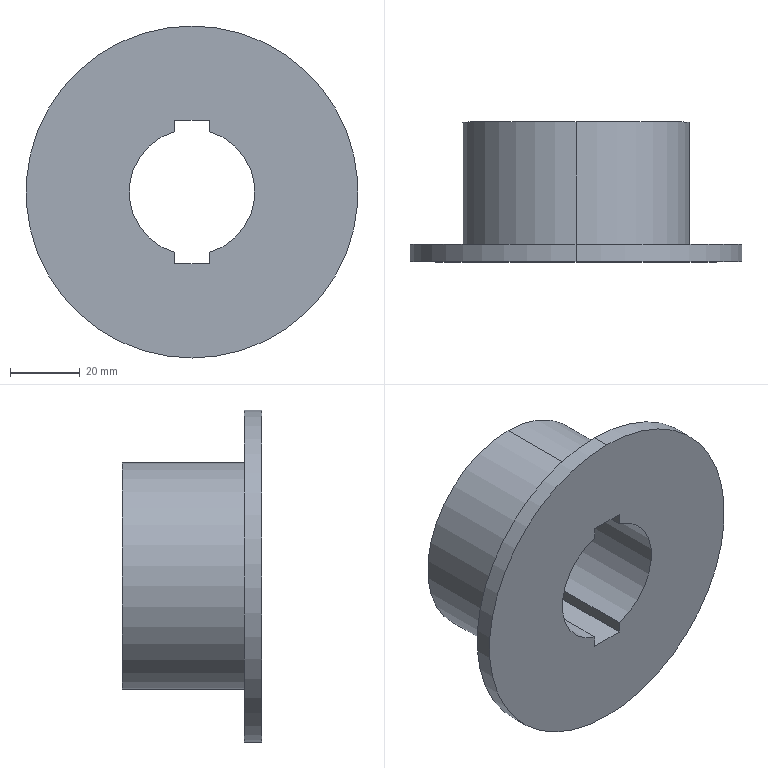Part | SolidWorks | features Extrusion 1, ICE 1 | 1 solid | 15 faces | box 95 x 40 x 95 mm | volume 108607 mm3 | plane 9 | cylinder 6 | commonest cylinder face diameters 36 x2 65 x2 95 x2
STEP:
#1=CARTESIAN_POINT('',(0.,5.,-47.5));
#2=VERTEX_POINT('',#1);
#3=CARTESIAN_POINT('',(0.,5.,47.5));
#4=VERTEX_POINT('',#3);
#5=CARTESIAN_POINT('',(0.,5.,0.));
#6=DIRECTION('',(0.,-1.,0.));
#7=DIRECTION('',(0.,0.,-1.));
#8=AXIS2_PLACEMENT_3D('',#5,#6,#7);
#9=CIRCLE('',#8,47.5);
#10=EDGE_CURVE('',#2,#4,#9,.T.);
#11=ORIENTED_EDGE('',*,*,#10,.T.);
#12=CARTESIAN_POINT('',(0.,0.,47.5));
#13=VERTEX_POINT('',#12);
#14=CARTESIAN_POINT('',(0.,5.,47.5));
#15=DIRECTION('',(0.,-1.,0.));
#16=VECTOR('',#15,1000.);
#17=LINE('',#14,#16);
#18=EDGE_CURVE('',#4,#13,#17,.T.);
#19=ORIENTED_EDGE('',*,*,#18,.T.);
#20=CARTESIAN_POINT('',(0.,0.,-47.5));
#21=VERTEX_POINT('',#20);
#22=CARTESIAN_POINT('',(0.,0.,0.));
#23=DIRECTION('',(0.,-1.,0.));
#24=DIRECTION('',(0.,0.,-1.));
#25=AXIS2_PLACEMENT_3D('',#22,#23,#24);
#26=CIRCLE('',#25,47.5);
#27=EDGE_CURVE('',#21,#13,#26,.T.);
#28=ORIENTED_EDGE('',*,*,#27,.F.);
#29=CARTESIAN_POINT('',(0.,5.,-47.5));
#30=DIRECTION('',(0.,-1.,0.));
#31=VECTOR('',#30,1000.);
#32=LINE('',#29,#31);
#33=EDGE_CURVE('',#2,#21,#32,.T.);
#34=ORIENTED_EDGE('',*,*,#33,.F.);
#35=EDGE_LOOP('',(#11,#19,#28,#34));
#36=FACE_OUTER_BOUND('',#35,.T.);
#37=CARTESIAN_POINT('',(0.,5.,0.));
#38=DIRECTION('',(0.,-1.,0.));
#39=DIRECTION('',(0.,0.,-1.));
#40=AXIS2_PLACEMENT_3D('',#37,#38,#39);
#41=CYLINDRICAL_SURFACE('',#40,47.5);
#42=ADVANCED_FACE('',(#36),#41,.T.);
#43=CARTESIAN_POINT('',(0.,40.,32.5));
#44=VERTEX_POINT('',#43);
#45=CARTESIAN_POINT('',(0.,40.,-32.5));
#46=VERTEX_POINT('',#45);
#47=CARTESIAN_POINT('',(0.,40.,0.));
#48=DIRECTION('',(0.,1.,0.));
#49=DIRECTION('',(0.,0.,1.));
#50=AXIS2_PLACEMENT_3D('',#47,#48,#49);
#51=CIRCLE('',#50,32.5);
#52=EDGE_CURVE('',#44,#46,#51,.T.);
#53=ORIENTED_EDGE('',*,*,#52,.F.);
#54=CARTESIAN_POINT('',(0.,5.,32.5));
#55=VERTEX_POINT('',#54);
#56=CARTESIAN_POINT('',(0.,40.,32.5));
#57=DIRECTION('',(0.,-1.,0.));
#58=VECTOR('',#57,1000.);
#59=LINE('',#56,#58);
#60=EDGE_CURVE('',#44,#55,#59,.T.);
#61=ORIENTED_EDGE('',*,*,#60,.T.);
#62=CARTESIAN_POINT('',(0.,5.,-32.5));
#63=VERTEX_POINT('',#62);
#64=CARTESIAN_POINT('',(0.,5.,0.));
#65=DIRECTION('',(0.,-1.,0.));
#66=DIRECTION('',(0.,0.,-1.));
#67=AXIS2_PLACEMENT_3D('',#64,#65,#66);
#68=CIRCLE('',#67,32.5);
#69=EDGE_CURVE('',#63,#55,#68,.T.);
#70=ORIENTED_EDGE('',*,*,#69,.F.);
#71=CARTESIAN_POINT('',(0.,40.,-32.5));
#72=DIRECTION('',(0.,-1.,0.));
#73=VECTOR('',#72,1000.);
#74=LINE('',#71,#73);
#75=EDGE_CURVE('',#46,#63,#74,.T.);
#76=ORIENTED_EDGE('',*,*,#75,.F.);
#77=EDGE_LOOP('',(#53,#61,#70,#76));
#78=FACE_OUTER_BOUND('',#77,.T.);
#79=CARTESIAN_POINT('',(0.,40.,0.));
#80=DIRECTION('',(0.,-1.,0.));
#81=DIRECTION('',(0.,0.,-1.));
#82=AXIS2_PLACEMENT_3D('',#79,#80,#81);
#83=CYLINDRICAL_SURFACE('',#82,32.5);
#84=ADVANCED_FACE('',(#78),#83,.T.);
#85=ORIENTED_EDGE('',*,*,#60,.F.);
#86=CARTESIAN_POINT('',(0.,40.,0.));
#87=DIRECTION('',(0.,1.,0.));
#88=DIRECTION('',(0.,0.,1.));
#89=AXIS2_PLACEMENT_3D('',#86,#87,#88);
#90=CIRCLE('',#89,32.5);
#91=EDGE_CURVE('',#46,#44,#90,.T.);
#92=ORIENTED_EDGE('',*,*,#91,.F.);
#93=ORIENTED_EDGE('',*,*,#75,.T.);
#94=CARTESIAN_POINT('',(0.,5.,0.));
#95=DIRECTION('',(0.,-1.,0.));
#96=DIRECTION('',(0.,0.,-1.));
#97=AXIS2_PLACEMENT_3D('',#94,#95,#96);
#98=CIRCLE('',#97,32.5);
#99=EDGE_CURVE('',#55,#63,#98,.T.);
#100=ORIENTED_EDGE('',*,*,#99,.F.);
#101=EDGE_LOOP('',(#85,#92,#93,#100));
#102=FACE_OUTER_BOUND('',#101,.T.);
#103=CARTESIAN_POINT('',(0.,40.,0.));
#104=DIRECTION('',(0.,-1.,0.));
#105=DIRECTION('',(0.,0.,-1.));
#106=AXIS2_PLACEMENT_3D('',#103,#104,#105);
#107=CYLINDRICAL_SURFACE('',#106,32.5);
#108=ADVANCED_FACE('',(#102),#107,.T.);
#109=ORIENTED_EDGE('',*,*,#91,.T.);
#110=ORIENTED_EDGE('',*,*,#52,.T.);
#111=EDGE_LOOP('',(#109,#110));
#112=FACE_OUTER_BOUND('',#111,.T.);
#113=CARTESIAN_POINT('',(-5.,40.,-17.292));
#114=VERTEX_POINT('',#113);
#115=CARTESIAN_POINT('',(-5.,40.,17.292));
#116=VERTEX_POINT('',#115);
#117=CARTESIAN_POINT('',(0.,40.,0.));
#118=DIRECTION('',(0.,1.,0.));
#119=DIRECTION('',(0.,0.,1.));
#120=AXIS2_PLACEMENT_3D('',#117,#118,#119);
#121=CIRCLE('',#120,18.);
#122=EDGE_CURVE('',#114,#116,#121,.T.);
#123=ORIENTED_EDGE('',*,*,#122,.F.);
#124=CARTESIAN_POINT('',(-5.,40.,-20.592));
#125=VERTEX_POINT('',#124);
#126=CARTESIAN_POINT('',(-5.,40.,-17.292));
#127=DIRECTION('',(0.,0.,1.));
#128=VECTOR('',#127,1000.);
#129=LINE('',#126,#128);
#130=EDGE_CURVE('',#125,#114,#129,.T.);
#131=ORIENTED_EDGE('',*,*,#130,.F.);
#132=CARTESIAN_POINT('',(5.,40.,-20.592));
#133=VERTEX_POINT('',#132);
#134=CARTESIAN_POINT('',(-5.,40.,-20.592));
#135=DIRECTION('',(-1.,0.,0.));
#136=VECTOR('',#135,1000.);
#137=LINE('',#134,#136);
#138=EDGE_CURVE('',#133,#125,#137,.T.);
#139=ORIENTED_EDGE('',*,*,#138,.F.);
#140=CARTESIAN_POINT('',(5.,40.,-17.292));
#141=VERTEX_POINT('',#140);
#142=CARTESIAN_POINT('',(5.,40.,-20.592));
#143=DIRECTION('',(0.,0.,-1.));
#144=VECTOR('',#143,1000.);
#145=LINE('',#142,#144);
#146=EDGE_CURVE('',#141,#133,#145,.T.);
#147=ORIENTED_EDGE('',*,*,#146,.F.);
#148=CARTESIAN_POINT('',(5.,40.,17.292));
#149=VERTEX_POINT('',#148);
#150=CARTESIAN_POINT('',(0.,40.,0.));
#151=DIRECTION('',(0.,1.,0.));
#152=DIRECTION('',(0.,0.,1.));
#153=AXIS2_PLACEMENT_3D('',#150,#151,#152);
#154=CIRCLE('',#153,18.);
#155=EDGE_CURVE('',#149,#141,#154,.T.);
#156=ORIENTED_EDGE('',*,*,#155,.F.);
#157=CARTESIAN_POINT('',(5.,40.,20.592));
#158=VERTEX_POINT('',#157);
#159=CARTESIAN_POINT('',(5.,40.,20.592));
#160=DIRECTION('',(0.,0.,-1.));
#161=VECTOR('',#160,1000.);
#162=LINE('',#159,#161);
#163=EDGE_CURVE('',#158,#149,#162,.T.);
#164=ORIENTED_EDGE('',*,*,#163,.F.);
#165=CARTESIAN_POINT('',(-5.,40.,20.592));
#166=VERTEX_POINT('',#165);
#167=CARTESIAN_POINT('',(-5.,40.,20.592));
#168=DIRECTION('',(1.,0.,0.));
#169=VECTOR('',#168,1000.);
#170=LINE('',#167,#169);
#171=EDGE_CURVE('',#166,#158,#170,.T.);
#172=ORIENTED_EDGE('',*,*,#171,.F.);
#173=CARTESIAN_POINT('',(-5.,40.,17.292));
#174=DIRECTION('',(0.,0.,1.));
#175=VECTOR('',#174,1000.);
#176=LINE('',#173,#175);
#177=EDGE_CURVE('',#116,#166,#176,.T.);
#178=ORIENTED_EDGE('',*,*,#177,.F.);
#179=EDGE_LOOP('',(#123,#131,#139,#147,#156,#164,#172,#178));
#180=FACE_BOUND('',#179,.T.);
#181=CARTESIAN_POINT('',(0.,40.,0.));
#182=DIRECTION('',(0.,1.,0.));
#183=DIRECTION('',(0.,0.,1.));
#184=AXIS2_PLACEMENT_3D('',#181,#182,#183);
#185=PLANE('',#184);
#186=ADVANCED_FACE('',(#112,#180),#185,.T.);
#187=ORIENTED_EDGE('',*,*,#27,.T.);
#188=CARTESIAN_POINT('',(0.,0.,0.));
#189=DIRECTION('',(0.,-1.,0.));
#190=DIRECTION('',(0.,0.,-1.));
#191=AXIS2_PLACEMENT_3D('',#188,#189,#190);
#192=CIRCLE('',#191,47.5);
#193=EDGE_CURVE('',#13,#21,#192,.T.);
#194=ORIENTED_EDGE('',*,*,#193,.T.);
#195=EDGE_LOOP('',(#187,#194));
#196=FACE_OUTER_BOUND('',#195,.T.);
#197=CARTESIAN_POINT('',(-5.,0.,-20.592));
#198=VERTEX_POINT('',#197);
#199=CARTESIAN_POINT('',(-5.,0.,-17.292));
#200=VERTEX_POINT('',#199);
#201=CARTESIAN_POINT('',(-5.,0.,-17.292));
#202=DIRECTION('',(0.,0.,1.));
#203=VECTOR('',#202,1000.);
#204=LINE('',#201,#203);
#205=EDGE_CURVE('',#198,#200,#204,.T.);
#206=ORIENTED_EDGE('',*,*,#205,.T.);
#207=CARTESIAN_POINT('',(-5.,0.,17.292));
#208=VERTEX_POINT('',#207);
#209=CARTESIAN_POINT('',(0.,0.,0.));
#210=DIRECTION('',(0.,1.,0.));
#211=DIRECTION('',(0.,0.,1.));
#212=AXIS2_PLACEMENT_3D('',#209,#210,#211);
#213=CIRCLE('',#212,18.);
#214=EDGE_CURVE('',#200,#208,#213,.T.);
#215=ORIENTED_EDGE('',*,*,#214,.T.);
#216=CARTESIAN_POINT('',(-5.,0.,20.592));
#217=VERTEX_POINT('',#216);
#218=CARTESIAN_POINT('',(-5.,0.,17.292));
#219=DIRECTION('',(0.,0.,1.));
#220=VECTOR('',#219,1000.);
#221=LINE('',#218,#220);
#222=EDGE_CURVE('',#208,#217,#221,.T.);
#223=ORIENTED_EDGE('',*,*,#222,.T.);
#224=CARTESIAN_POINT('',(5.,0.,20.592));
#225=VERTEX_POINT('',#224);
#226=CARTESIAN_POINT('',(0.,0.,20.592));
#227=DIRECTION('',(1.,0.,0.));
#228=VECTOR('',#227,1000.);
#229=LINE('',#226,#228);
#230=EDGE_CURVE('',#217,#225,#229,.T.);
#231=ORIENTED_EDGE('',*,*,#230,.T.);
#232=CARTESIAN_POINT('',(5.,0.,17.292));
#233=VERTEX_POINT('',#232);
#234=CARTESIAN_POINT('',(5.,0.,20.592));
#235=DIRECTION('',(0.,0.,-1.));
#236=VECTOR('',#235,1000.);
#237=LINE('',#234,#236);
#238=EDGE_CURVE('',#225,#233,#237,.T.);
#239=ORIENTED_EDGE('',*,*,#238,.T.);
#240=CARTESIAN_POINT('',(5.,0.,-17.292));
#241=VERTEX_POINT('',#240);
#242=CARTESIAN_POINT('',(0.,0.,0.));
#243=DIRECTION('',(0.,1.,0.));
#244=DIRECTION('',(0.,0.,1.));
#245=AXIS2_PLACEMENT_3D('',#242,#243,#244);
#246=CIRCLE('',#245,18.);
#247=EDGE_CURVE('',#233,#241,#246,.T.);
#248=ORIENTED_EDGE('',*,*,#247,.T.);
#249=CARTESIAN_POINT('',(5.,0.,-20.592));
#250=VERTEX_POINT('',#249);
#251=CARTESIAN_POINT('',(5.,0.,-20.592));
#252=DIRECTION('',(0.,0.,-1.));
#253=VECTOR('',#252,1000.);
#254=LINE('',#251,#253);
#255=EDGE_CURVE('',#241,#250,#254,.T.);
#256=ORIENTED_EDGE('',*,*,#255,.T.);
#257=CARTESIAN_POINT('',(0.,0.,-20.592));
#258=DIRECTION('',(-1.,0.,0.));
#259=VECTOR('',#258,1000.);
#260=LINE('',#257,#259);
#261=EDGE_CURVE('',#250,#198,#260,.T.);
#262=ORIENTED_EDGE('',*,*,#261,.T.);
#263=EDGE_LOOP('',(#206,#215,#223,#231,#239,#248,#256,#262));
#264=FACE_BOUND('',#263,.T.);
#265=CARTESIAN_POINT('',(0.,0.,0.));
#266=DIRECTION('',(0.,1.,0.));
#267=DIRECTION('',(0.,0.,1.));
#268=AXIS2_PLACEMENT_3D('',#265,#266,#267);
#269=PLANE('',#268);
#270=ADVANCED_FACE('',(#196,#264),#269,.F.);
#271=ORIENTED_EDGE('',*,*,#205,.F.);
#272=CARTESIAN_POINT('',(-5.,40.,-20.592));
#273=DIRECTION('',(0.,-1.,0.));
#274=VECTOR('',#273,1000.);
#275=LINE('',#272,#274);
#276=EDGE_CURVE('',#125,#198,#275,.T.);
#277=ORIENTED_EDGE('',*,*,#276,.F.);
#278=ORIENTED_EDGE('',*,*,#130,.T.);
#279=CARTESIAN_POINT('',(-5.,40.,-17.292));
#280=DIRECTION('',(0.,-1.,0.));
#281=VECTOR('',#280,1000.);
#282=LINE('',#279,#281);
#283=EDGE_CURVE('',#114,#200,#282,.T.);
#284=ORIENTED_EDGE('',*,*,#283,.T.);
#285=EDGE_LOOP('',(#271,#277,#278,#284));
#286=FACE_OUTER_BOUND('',#285,.T.);
#287=CARTESIAN_POINT('',(-5.,40.,-17.292));
#288=DIRECTION('',(1.,0.,0.));
#289=DIRECTION('',(0.,0.,-1.));
#290=AXIS2_PLACEMENT_3D('',#287,#288,#289);
#291=PLANE('',#290);
#292=ADVANCED_FACE('',(#286),#291,.T.);
#293=ORIENTED_EDGE('',*,*,#214,.F.);
#294=ORIENTED_EDGE('',*,*,#283,.F.);
#295=ORIENTED_EDGE('',*,*,#122,.T.);
#296=CARTESIAN_POINT('',(-5.,40.,17.292));
#297=DIRECTION('',(0.,-1.,0.));
#298=VECTOR('',#297,1000.);
#299=LINE('',#296,#298);
#300=EDGE_CURVE('',#116,#208,#299,.T.);
#301=ORIENTED_EDGE('',*,*,#300,.T.);
#302=EDGE_LOOP('',(#293,#294,#295,#301));
#303=FACE_OUTER_BOUND('',#302,.T.);
#304=CARTESIAN_POINT('',(0.,40.,0.));
#305=DIRECTION('',(0.,-1.,0.));
#306=DIRECTION('',(0.,0.,-1.));
#307=AXIS2_PLACEMENT_3D('',#304,#305,#306);
#308=CYLINDRICAL_SURFACE('',#307,18.);
#309=ADVANCED_FACE('',(#303),#308,.F.);
#310=ORIENTED_EDGE('',*,*,#222,.F.);
#311=ORIENTED_EDGE('',*,*,#300,.F.);
#312=ORIENTED_EDGE('',*,*,#177,.T.);
#313=CARTESIAN_POINT('',(-5.,40.,20.592));
#314=DIRECTION('',(0.,-1.,0.));
#315=VECTOR('',#314,1000.);
#316=LINE('',#313,#315);
#317=EDGE_CURVE('',#166,#217,#316,.T.);
#318=ORIENTED_EDGE('',*,*,#317,.T.);
#319=EDGE_LOOP('',(#310,#311,#312,#318));
#320=FACE_OUTER_BOUND('',#319,.T.);
#321=CARTESIAN_POINT('',(-5.,40.,17.292));
#322=DIRECTION('',(1.,0.,0.));
#323=DIRECTION('',(0.,0.,-1.));
#324=AXIS2_PLACEMENT_3D('',#321,#322,#323);
#325=PLANE('',#324);
#326=ADVANCED_FACE('',(#320),#325,.T.);
#327=ORIENTED_EDGE('',*,*,#230,.F.);
#328=ORIENTED_EDGE('',*,*,#317,.F.);
#329=ORIENTED_EDGE('',*,*,#171,.T.);
#330=CARTESIAN_POINT('',(5.,40.,20.592));
#331=DIRECTION('',(0.,-1.,0.));
#332=VECTOR('',#331,1000.);
#333=LINE('',#330,#332);
#334=EDGE_CURVE('',#158,#225,#333,.T.);
#335=ORIENTED_EDGE('',*,*,#334,.T.);
#336=EDGE_LOOP('',(#327,#328,#329,#335));
#337=FACE_OUTER_BOUND('',#336,.T.);
#338=CARTESIAN_POINT('',(0.,40.,20.592));
#339=DIRECTION('',(0.,0.,-1.));
#340=DIRECTION('',(-1.,0.,0.));
#341=AXIS2_PLACEMENT_3D('',#338,#339,#340);
#342=PLANE('',#341);
#343=ADVANCED_FACE('',(#337),#342,.T.);
#344=ORIENTED_EDGE('',*,*,#238,.F.);
#345=ORIENTED_EDGE('',*,*,#334,.F.);
#346=ORIENTED_EDGE('',*,*,#163,.T.);
#347=CARTESIAN_POINT('',(5.,40.,17.292));
#348=DIRECTION('',(0.,-1.,0.));
#349=VECTOR('',#348,1000.);
#350=LINE('',#347,#349);
#351=EDGE_CURVE('',#149,#233,#350,.T.);
#352=ORIENTED_EDGE('',*,*,#351,.T.);
#353=EDGE_LOOP('',(#344,#345,#346,#352));
#354=FACE_OUTER_BOUND('',#353,.T.);
#355=CARTESIAN_POINT('',(5.,40.,20.592));
#356=DIRECTION('',(-1.,0.,0.));
#357=DIRECTION('',(0.,0.,1.));
#358=AXIS2_PLACEMENT_3D('',#355,#356,#357);
#359=PLANE('',#358);
#360=ADVANCED_FACE('',(#354),#359,.T.);
#361=ORIENTED_EDGE('',*,*,#247,.F.);
#362=ORIENTED_EDGE('',*,*,#351,.F.);
#363=ORIENTED_EDGE('',*,*,#155,.T.);
#364=CARTESIAN_POINT('',(5.,40.,-17.292));
#365=DIRECTION('',(0.,-1.,0.));
#366=VECTOR('',#365,1000.);
#367=LINE('',#364,#366);
#368=EDGE_CURVE('',#141,#241,#367,.T.);
#369=ORIENTED_EDGE('',*,*,#368,.T.);
#370=EDGE_LOOP('',(#361,#362,#363,#369));
#371=FACE_OUTER_BOUND('',#370,.T.);
#372=CARTESIAN_POINT('',(0.,40.,0.));
#373=DIRECTION('',(0.,-1.,0.));
#374=DIRECTION('',(0.,0.,-1.));
#375=AXIS2_PLACEMENT_3D('',#372,#373,#374);
#376=CYLINDRICAL_SURFACE('',#375,18.);
#377=ADVANCED_FACE('',(#371),#376,.F.);
#378=ORIENTED_EDGE('',*,*,#255,.F.);
#379=ORIENTED_EDGE('',*,*,#368,.F.);
#380=ORIENTED_EDGE('',*,*,#146,.T.);
#381=CARTESIAN_POINT('',(5.,40.,-20.592));
#382=DIRECTION('',(0.,-1.,0.));
#383=VECTOR('',#382,1000.);
#384=LINE('',#381,#383);
#385=EDGE_CURVE('',#133,#250,#384,.T.);
#386=ORIENTED_EDGE('',*,*,#385,.T.);
#387=EDGE_LOOP('',(#378,#379,#380,#386));
#388=FACE_OUTER_BOUND('',#387,.T.);
#389=CARTESIAN_POINT('',(5.,40.,-20.592));
#390=DIRECTION('',(-1.,0.,0.));
#391=DIRECTION('',(0.,0.,1.));
#392=AXIS2_PLACEMENT_3D('',#389,#390,#391);
#393=PLANE('',#392);
#394=ADVANCED_FACE('',(#388),#393,.T.);
#395=ORIENTED_EDGE('',*,*,#261,.F.);
#396=ORIENTED_EDGE('',*,*,#385,.F.);
#397=ORIENTED_EDGE('',*,*,#138,.T.);
#398=ORIENTED_EDGE('',*,*,#276,.T.);
#399=EDGE_LOOP('',(#395,#396,#397,#398));
#400=FACE_OUTER_BOUND('',#399,.T.);
#401=CARTESIAN_POINT('',(0.,40.,-20.592));
#402=DIRECTION('',(0.,0.,1.));
#403=DIRECTION('',(1.,0.,0.));
#404=AXIS2_PLACEMENT_3D('',#401,#402,#403);
#405=PLANE('',#404);
#406=ADVANCED_FACE('',(#400),#405,.T.);
#407=ORIENTED_EDGE('',*,*,#10,.F.);
#408=CARTESIAN_POINT('',(0.,5.,0.));
#409=DIRECTION('',(0.,-1.,0.));
#410=DIRECTION('',(0.,0.,-1.));
#411=AXIS2_PLACEMENT_3D('',#408,#409,#410);
#412=CIRCLE('',#411,47.5);
#413=EDGE_CURVE('',#4,#2,#412,.T.);
#414=ORIENTED_EDGE('',*,*,#413,.F.);
#415=EDGE_LOOP('',(#407,#414));
#416=FACE_OUTER_BOUND('',#415,.T.);
#417=ORIENTED_EDGE('',*,*,#69,.T.);
#418=ORIENTED_EDGE('',*,*,#99,.T.);
#419=EDGE_LOOP('',(#417,#418));
#420=FACE_BOUND('',#419,.T.);
#421=CARTESIAN_POINT('',(0.,5.,0.));
#422=DIRECTION('',(0.,-1.,0.));
#423=DIRECTION('',(0.,0.,-1.));
#424=AXIS2_PLACEMENT_3D('',#421,#422,#423);
#425=PLANE('',#424);
#426=ADVANCED_FACE('',(#416,#420),#425,.F.);
#427=ORIENTED_EDGE('',*,*,#18,.F.);
#428=ORIENTED_EDGE('',*,*,#413,.T.);
#429=ORIENTED_EDGE('',*,*,#33,.T.);
#430=ORIENTED_EDGE('',*,*,#193,.F.);
#431=EDGE_LOOP('',(#427,#428,#429,#430));
#432=FACE_OUTER_BOUND('',#431,.T.);
#433=CARTESIAN_POINT('',(0.,5.,0.));
#434=DIRECTION('',(0.,-1.,0.));
#435=DIRECTION('',(0.,0.,-1.));
#436=AXIS2_PLACEMENT_3D('',#433,#434,#435);
#437=CYLINDRICAL_SURFACE('',#436,47.5);
#438=ADVANCED_FACE('',(#432),#437,.T.);
#439=CLOSED_SHELL('',(#42,#84,#108,#186,#270,#292,#309,#326,#343,#360,#377,#394,#406,#426,#438));
#440=MANIFOLD_SOLID_BREP('',#439);
#441=CARTESIAN_POINT('',(0.,0.,0.));
#442=DIRECTION('',(0.,0.,1.));
#443=DIRECTION('',(1.,0.,0.));
#444=AXIS2_PLACEMENT_3D('',#441,#442,#443);
#445=(LENGTH_UNIT()NAMED_UNIT(*)SI_UNIT(.MILLI.,.METRE.));
#446=UNCERTAINTY_MEASURE_WITH_UNIT(LENGTH_MEASURE(0.00001),#445,'','');
#447=(NAMED_UNIT(*)PLANE_ANGLE_UNIT()SI_UNIT($,.RADIAN.));
#448=(NAMED_UNIT(*)SI_UNIT($,.STERADIAN.)SOLID_ANGLE_UNIT());
#449=(GEOMETRIC_REPRESENTATION_CONTEXT(3)GLOBAL_UNCERTAINTY_ASSIGNED_CONTEXT((#446))GLOBAL_UNIT_ASSIGNED_CONTEXT((#445,#447,#448))REPRESENTATION_CONTEXT('',''));
#450=ADVANCED_BREP_SHAPE_REPRESENTATION('',(#440,#444),#449);